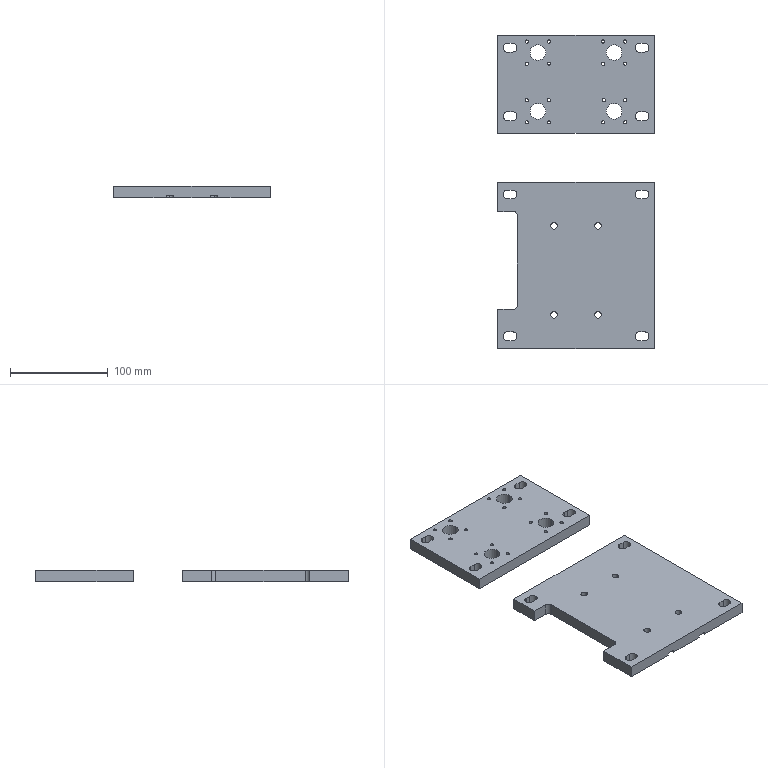Part | STEP file | X77b-01006 | 2 solids | 116 faces | box 160 x 320 x 12 mm | volume 465416 mm3 | cylinder 78 | plane 38 | commonest cylinder face diameters 3.3 x32 9 x24 6.8 x8 16 x8 8 x6